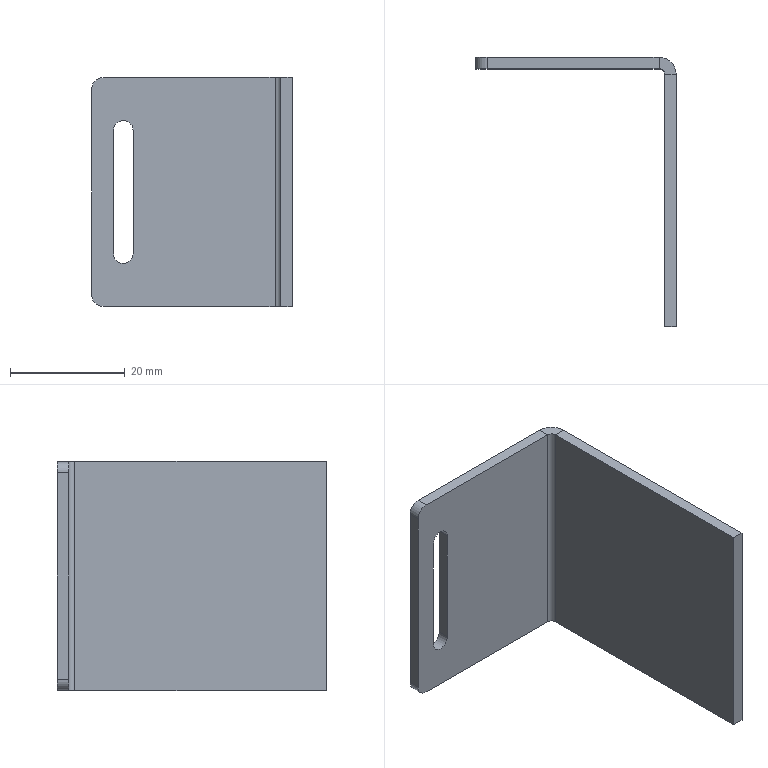Part | NX | features BREP 1 | 1 solid | 21 faces | box 35 x 47 x 40 mm | volume 6163 mm3 | plane 14 | cylinder 7 | commonest cylinder face diameters 3.4 x3 4 x2 2 x1 6 x1
STEP:
#1=CARTESIAN_POINT('',(2.,-2.,20.));
#2=VERTEX_POINT('',#1);
#3=CARTESIAN_POINT('',(0.,-2.,18.));
#4=VERTEX_POINT('',#3);
#5=CARTESIAN_POINT('',(2.,-2.,18.));
#6=DIRECTION('',(0.,-1.,0.));
#7=DIRECTION('',(0.,0.,1.));
#8=AXIS2_PLACEMENT_3D('',#5,#6,#7);
#9=CIRCLE('',#8,2.);
#10=EDGE_CURVE('',#2,#4,#9,.T.);
#11=ORIENTED_EDGE('',*,*,#10,.F.);
#12=CARTESIAN_POINT('',(2.,0.,20.));
#13=VERTEX_POINT('',#12);
#14=CARTESIAN_POINT('',(2.,-3.,20.));
#15=DIRECTION('',(0.,-1.,0.));
#16=VECTOR('',#15,1000.);
#17=LINE('',#14,#16);
#18=EDGE_CURVE('',#13,#2,#17,.T.);
#19=ORIENTED_EDGE('',*,*,#18,.F.);
#20=CARTESIAN_POINT('',(0.,0.,18.));
#21=VERTEX_POINT('',#20);
#22=CARTESIAN_POINT('',(2.,0.,18.));
#23=DIRECTION('',(0.,1.,0.));
#24=DIRECTION('',(0.,0.,1.));
#25=AXIS2_PLACEMENT_3D('',#22,#23,#24);
#26=CIRCLE('',#25,2.);
#27=EDGE_CURVE('',#21,#13,#26,.T.);
#28=ORIENTED_EDGE('',*,*,#27,.F.);
#29=CARTESIAN_POINT('',(0.,-2.,18.));
#30=DIRECTION('',(0.,1.,0.));
#31=VECTOR('',#30,1000.);
#32=LINE('',#29,#31);
#33=EDGE_CURVE('',#4,#21,#32,.T.);
#34=ORIENTED_EDGE('',*,*,#33,.F.);
#35=EDGE_LOOP('',(#11,#19,#28,#34));
#36=FACE_BOUND('',#35,.T.);
#37=CARTESIAN_POINT('',(2.,-2.,18.));
#38=DIRECTION('',(0.,1.,0.));
#39=DIRECTION('',(0.,0.,1.));
#40=AXIS2_PLACEMENT_3D('',#37,#38,#39);
#41=CYLINDRICAL_SURFACE('',#40,2.);
#42=ADVANCED_FACE('',(#36),#41,.T.);
#43=CARTESIAN_POINT('',(0.,-2.,-18.));
#44=VERTEX_POINT('',#43);
#45=CARTESIAN_POINT('',(2.,-2.,-20.));
#46=VERTEX_POINT('',#45);
#47=CARTESIAN_POINT('',(2.,-2.,-18.));
#48=DIRECTION('',(0.,-1.,0.));
#49=DIRECTION('',(0.,0.,1.));
#50=AXIS2_PLACEMENT_3D('',#47,#48,#49);
#51=CIRCLE('',#50,2.);
#52=EDGE_CURVE('',#44,#46,#51,.T.);
#53=ORIENTED_EDGE('',*,*,#52,.F.);
#54=CARTESIAN_POINT('',(0.,0.,-18.));
#55=VERTEX_POINT('',#54);
#56=CARTESIAN_POINT('',(0.,-2.,-18.));
#57=DIRECTION('',(0.,-1.,0.));
#58=VECTOR('',#57,1000.);
#59=LINE('',#56,#58);
#60=EDGE_CURVE('',#55,#44,#59,.T.);
#61=ORIENTED_EDGE('',*,*,#60,.F.);
#62=CARTESIAN_POINT('',(2.,0.,-20.));
#63=VERTEX_POINT('',#62);
#64=CARTESIAN_POINT('',(2.,0.,-18.));
#65=DIRECTION('',(0.,1.,0.));
#66=DIRECTION('',(0.,0.,1.));
#67=AXIS2_PLACEMENT_3D('',#64,#65,#66);
#68=CIRCLE('',#67,2.);
#69=EDGE_CURVE('',#63,#55,#68,.T.);
#70=ORIENTED_EDGE('',*,*,#69,.F.);
#71=CARTESIAN_POINT('',(2.,-3.,-20.));
#72=DIRECTION('',(0.,1.,0.));
#73=VECTOR('',#72,1000.);
#74=LINE('',#71,#73);
#75=EDGE_CURVE('',#46,#63,#74,.T.);
#76=ORIENTED_EDGE('',*,*,#75,.F.);
#77=EDGE_LOOP('',(#53,#61,#70,#76));
#78=FACE_BOUND('',#77,.T.);
#79=CARTESIAN_POINT('',(2.,-3.,-18.));
#80=DIRECTION('',(0.,1.,0.));
#81=DIRECTION('',(0.,0.,1.));
#82=AXIS2_PLACEMENT_3D('',#79,#80,#81);
#83=CYLINDRICAL_SURFACE('',#82,2.);
#84=ADVANCED_FACE('',(#78),#83,.T.);
#85=CARTESIAN_POINT('',(7.2,0.,-10.8));
#86=VERTEX_POINT('',#85);
#87=CARTESIAN_POINT('',(7.2,-2.,-10.8));
#88=VERTEX_POINT('',#87);
#89=CARTESIAN_POINT('',(7.2,-47.,-10.8));
#90=DIRECTION('',(0.,-1.,0.));
#91=VECTOR('',#90,1000.);
#92=LINE('',#89,#91);
#93=EDGE_CURVE('',#86,#88,#92,.T.);
#94=ORIENTED_EDGE('',*,*,#93,.F.);
#95=CARTESIAN_POINT('',(3.8,0.,-10.8));
#96=VERTEX_POINT('',#95);
#97=CARTESIAN_POINT('',(5.5,0.,-10.8));
#98=DIRECTION('',(0.,1.,0.));
#99=DIRECTION('',(0.,0.,1.));
#100=AXIS2_PLACEMENT_3D('',#97,#98,#99);
#101=CIRCLE('',#100,1.7);
#102=EDGE_CURVE('',#86,#96,#101,.T.);
#103=ORIENTED_EDGE('',*,*,#102,.T.);
#104=CARTESIAN_POINT('',(3.8,-2.,-10.8));
#105=VERTEX_POINT('',#104);
#106=CARTESIAN_POINT('',(3.8,0.,-10.8));
#107=DIRECTION('',(0.,1.,0.));
#108=VECTOR('',#107,1000.);
#109=LINE('',#106,#108);
#110=EDGE_CURVE('',#105,#96,#109,.T.);
#111=ORIENTED_EDGE('',*,*,#110,.F.);
#112=CARTESIAN_POINT('',(5.5,-2.,-10.8));
#113=DIRECTION('',(0.,1.,0.));
#114=DIRECTION('',(0.,0.,1.));
#115=AXIS2_PLACEMENT_3D('',#112,#113,#114);
#116=CIRCLE('',#115,1.7);
#117=EDGE_CURVE('',#88,#105,#116,.T.);
#118=ORIENTED_EDGE('',*,*,#117,.F.);
#119=EDGE_LOOP('',(#94,#103,#111,#118));
#120=FACE_BOUND('',#119,.T.);
#121=CARTESIAN_POINT('',(5.5,0.,-10.8));
#122=DIRECTION('',(0.,1.,0.));
#123=DIRECTION('',(0.,0.,1.));
#124=AXIS2_PLACEMENT_3D('',#121,#122,#123);
#125=CYLINDRICAL_SURFACE('',#124,1.7);
#126=ADVANCED_FACE('',(#120),#125,.F.);
#127=CARTESIAN_POINT('',(7.2,0.,10.8));
#128=VERTEX_POINT('',#127);
#129=CARTESIAN_POINT('',(7.2,-2.,10.8));
#130=VERTEX_POINT('',#129);
#131=CARTESIAN_POINT('',(7.2,-47.,10.8));
#132=DIRECTION('',(0.,-1.,0.));
#133=VECTOR('',#132,1000.);
#134=LINE('',#131,#133);
#135=EDGE_CURVE('',#128,#130,#134,.T.);
#136=ORIENTED_EDGE('',*,*,#135,.F.);
#137=CARTESIAN_POINT('',(7.2,0.,10.8));
#138=DIRECTION('',(0.,0.,-1.));
#139=VECTOR('',#138,1000.);
#140=LINE('',#137,#139);
#141=EDGE_CURVE('',#128,#86,#140,.T.);
#142=ORIENTED_EDGE('',*,*,#141,.T.);
#143=ORIENTED_EDGE('',*,*,#93,.T.);
#144=CARTESIAN_POINT('',(7.2,-2.,20.));
#145=DIRECTION('',(0.,0.,-1.));
#146=VECTOR('',#145,1000.);
#147=LINE('',#144,#146);
#148=EDGE_CURVE('',#130,#88,#147,.T.);
#149=ORIENTED_EDGE('',*,*,#148,.F.);
#150=EDGE_LOOP('',(#136,#142,#143,#149));
#151=FACE_BOUND('',#150,.T.);
#152=CARTESIAN_POINT('',(7.2,-47.,10.8));
#153=DIRECTION('',(1.,0.,0.));
#154=DIRECTION('',(0.,1.,0.));
#155=AXIS2_PLACEMENT_3D('',#152,#153,#154);
#156=PLANE('',#155);
#157=ADVANCED_FACE('',(#151),#156,.F.);
#158=CARTESIAN_POINT('',(5.5,-2.,12.5));
#159=VERTEX_POINT('',#158);
#160=CARTESIAN_POINT('',(5.5,0.,12.5));
#161=VERTEX_POINT('',#160);
#162=CARTESIAN_POINT('',(5.5,0.,12.5));
#163=DIRECTION('',(0.,1.,0.));
#164=VECTOR('',#163,1000.);
#165=LINE('',#162,#164);
#166=EDGE_CURVE('',#159,#161,#165,.T.);
#167=ORIENTED_EDGE('',*,*,#166,.F.);
#168=CARTESIAN_POINT('',(3.8,-2.,10.8));
#169=VERTEX_POINT('',#168);
#170=CARTESIAN_POINT('',(5.5,-2.,10.8));
#171=DIRECTION('',(0.,1.,0.));
#172=DIRECTION('',(0.,0.,1.));
#173=AXIS2_PLACEMENT_3D('',#170,#171,#172);
#174=CIRCLE('',#173,1.7);
#175=EDGE_CURVE('',#169,#159,#174,.T.);
#176=ORIENTED_EDGE('',*,*,#175,.F.);
#177=CARTESIAN_POINT('',(3.8,0.,10.8));
#178=VERTEX_POINT('',#177);
#179=CARTESIAN_POINT('',(3.8,0.,10.8));
#180=DIRECTION('',(0.,-1.,0.));
#181=VECTOR('',#180,1000.);
#182=LINE('',#179,#181);
#183=EDGE_CURVE('',#178,#169,#182,.T.);
#184=ORIENTED_EDGE('',*,*,#183,.F.);
#185=CARTESIAN_POINT('',(5.5,0.,10.8));
#186=DIRECTION('',(0.,1.,0.));
#187=DIRECTION('',(0.,0.,1.));
#188=AXIS2_PLACEMENT_3D('',#185,#186,#187);
#189=CIRCLE('',#188,1.7);
#190=EDGE_CURVE('',#178,#161,#189,.T.);
#191=ORIENTED_EDGE('',*,*,#190,.T.);
#192=EDGE_LOOP('',(#167,#176,#184,#191));
#193=FACE_BOUND('',#192,.T.);
#194=CARTESIAN_POINT('',(5.5,0.,10.8));
#195=DIRECTION('',(0.,1.,0.));
#196=DIRECTION('',(0.,0.,1.));
#197=AXIS2_PLACEMENT_3D('',#194,#195,#196);
#198=CYLINDRICAL_SURFACE('',#197,1.7);
#199=ADVANCED_FACE('',(#193),#198,.F.);
#200=ORIENTED_EDGE('',*,*,#110,.T.);
#201=CARTESIAN_POINT('',(3.8,0.,10.8));
#202=DIRECTION('',(0.,0.,-1.));
#203=VECTOR('',#202,1000.);
#204=LINE('',#201,#203);
#205=EDGE_CURVE('',#178,#96,#204,.T.);
#206=ORIENTED_EDGE('',*,*,#205,.F.);
#207=ORIENTED_EDGE('',*,*,#183,.T.);
#208=CARTESIAN_POINT('',(3.8,-2.,20.));
#209=DIRECTION('',(0.,0.,1.));
#210=VECTOR('',#209,1000.);
#211=LINE('',#208,#210);
#212=EDGE_CURVE('',#105,#169,#211,.T.);
#213=ORIENTED_EDGE('',*,*,#212,.F.);
#214=EDGE_LOOP('',(#200,#206,#207,#213));
#215=FACE_BOUND('',#214,.T.);
#216=CARTESIAN_POINT('',(3.8,0.,10.8));
#217=DIRECTION('',(-1.,0.,0.));
#218=DIRECTION('',(0.,0.,1.));
#219=AXIS2_PLACEMENT_3D('',#216,#217,#218);
#220=PLANE('',#219);
#221=ADVANCED_FACE('',(#215),#220,.F.);
#222=CARTESIAN_POINT('',(33.,-3.,-20.));
#223=VERTEX_POINT('',#222);
#224=CARTESIAN_POINT('',(33.,-47.,-20.));
#225=VERTEX_POINT('',#224);
#226=CARTESIAN_POINT('',(33.,0.,-20.));
#227=DIRECTION('',(0.,-1.,0.));
#228=VECTOR('',#227,1000.);
#229=LINE('',#226,#228);
#230=EDGE_CURVE('',#223,#225,#229,.T.);
#231=ORIENTED_EDGE('',*,*,#230,.F.);
#232=CARTESIAN_POINT('',(35.,-3.,-20.));
#233=VERTEX_POINT('',#232);
#234=CARTESIAN_POINT('',(33.,-3.,-20.));
#235=DIRECTION('',(1.,0.,0.));
#236=VECTOR('',#235,1000.);
#237=LINE('',#234,#236);
#238=EDGE_CURVE('',#223,#233,#237,.T.);
#239=ORIENTED_EDGE('',*,*,#238,.T.);
#240=CARTESIAN_POINT('',(35.,-47.,-20.));
#241=VERTEX_POINT('',#240);
#242=CARTESIAN_POINT('',(35.,0.,-20.));
#243=DIRECTION('',(0.,-1.,0.));
#244=VECTOR('',#243,1000.);
#245=LINE('',#242,#244);
#246=EDGE_CURVE('',#233,#241,#245,.T.);
#247=ORIENTED_EDGE('',*,*,#246,.T.);
#248=CARTESIAN_POINT('',(35.,-47.,-20.));
#249=DIRECTION('',(-1.,0.,0.));
#250=VECTOR('',#249,1000.);
#251=LINE('',#248,#250);
#252=EDGE_CURVE('',#241,#225,#251,.T.);
#253=ORIENTED_EDGE('',*,*,#252,.T.);
#254=EDGE_LOOP('',(#231,#239,#247,#253));
#255=FACE_BOUND('',#254,.T.);
#256=CARTESIAN_POINT('',(32.,-3.,-20.));
#257=DIRECTION('',(0.,0.,1.));
#258=DIRECTION('',(1.,0.,0.));
#259=AXIS2_PLACEMENT_3D('',#256,#257,#258);
#260=PLANE('',#259);
#261=ADVANCED_FACE('',(#255),#260,.F.);
#262=CARTESIAN_POINT('',(32.,0.,20.));
#263=VERTEX_POINT('',#262);
#264=CARTESIAN_POINT('',(0.,0.,20.));
#265=DIRECTION('',(1.,0.,0.));
#266=VECTOR('',#265,1000.);
#267=LINE('',#264,#266);
#268=EDGE_CURVE('',#13,#263,#267,.T.);
#269=ORIENTED_EDGE('',*,*,#268,.F.);
#270=ORIENTED_EDGE('',*,*,#18,.T.);
#271=CARTESIAN_POINT('',(32.,-2.,20.));
#272=VERTEX_POINT('',#271);
#273=CARTESIAN_POINT('',(0.,-2.,20.));
#274=DIRECTION('',(1.,0.,0.));
#275=VECTOR('',#274,1000.);
#276=LINE('',#273,#275);
#277=EDGE_CURVE('',#2,#272,#276,.T.);
#278=ORIENTED_EDGE('',*,*,#277,.T.);
#279=CARTESIAN_POINT('',(32.,-2.,20.));
#280=DIRECTION('',(0.,1.,0.));
#281=VECTOR('',#280,1000.);
#282=LINE('',#279,#281);
#283=EDGE_CURVE('',#272,#263,#282,.T.);
#284=ORIENTED_EDGE('',*,*,#283,.T.);
#285=EDGE_LOOP('',(#269,#270,#278,#284));
#286=FACE_BOUND('',#285,.T.);
#287=CARTESIAN_POINT('',(32.,-3.,20.));
#288=DIRECTION('',(0.,0.,1.));
#289=DIRECTION('',(1.,0.,0.));
#290=AXIS2_PLACEMENT_3D('',#287,#288,#289);
#291=PLANE('',#290);
#292=ADVANCED_FACE('',(#286),#291,.T.);
#293=CARTESIAN_POINT('',(32.,-2.,-20.));
#294=VERTEX_POINT('',#293);
#295=CARTESIAN_POINT('',(32.,-3.,-20.));
#296=DIRECTION('',(0.,0.,-1.));
#297=DIRECTION('',(1.,0.,0.));
#298=AXIS2_PLACEMENT_3D('',#295,#296,#297);
#299=CIRCLE('',#298,1.);
#300=EDGE_CURVE('',#294,#223,#299,.T.);
#301=ORIENTED_EDGE('',*,*,#300,.T.);
#302=CARTESIAN_POINT('',(33.,-3.,20.));
#303=VERTEX_POINT('',#302);
#304=CARTESIAN_POINT('',(33.,-3.,20.));
#305=DIRECTION('',(0.,0.,-1.));
#306=VECTOR('',#305,1000.);
#307=LINE('',#304,#306);
#308=EDGE_CURVE('',#303,#223,#307,.T.);
#309=ORIENTED_EDGE('',*,*,#308,.F.);
#310=CARTESIAN_POINT('',(32.,-3.,20.));
#311=DIRECTION('',(0.,0.,-1.));
#312=DIRECTION('',(1.,0.,0.));
#313=AXIS2_PLACEMENT_3D('',#310,#311,#312);
#314=CIRCLE('',#313,1.);
#315=EDGE_CURVE('',#272,#303,#314,.T.);
#316=ORIENTED_EDGE('',*,*,#315,.F.);
#317=CARTESIAN_POINT('',(32.,-2.,20.));
#318=DIRECTION('',(0.,0.,-1.));
#319=VECTOR('',#318,1000.);
#320=LINE('',#317,#319);
#321=EDGE_CURVE('',#272,#294,#320,.T.);
#322=ORIENTED_EDGE('',*,*,#321,.T.);
#323=EDGE_LOOP('',(#301,#309,#316,#322));
#324=FACE_BOUND('',#323,.T.);
#325=CARTESIAN_POINT('',(32.,-3.,20.));
#326=DIRECTION('',(0.,0.,-1.));
#327=DIRECTION('',(-1.,0.,0.));
#328=AXIS2_PLACEMENT_3D('',#325,#326,#327);
#329=CYLINDRICAL_SURFACE('',#328,1.);
#330=ADVANCED_FACE('',(#324),#329,.F.);
#331=CARTESIAN_POINT('',(0.,-2.,20.));
#332=DIRECTION('',(0.,0.,-1.));
#333=VECTOR('',#332,1000.);
#334=LINE('',#331,#333);
#335=EDGE_CURVE('',#4,#44,#334,.T.);
#336=ORIENTED_EDGE('',*,*,#335,.T.);
#337=ORIENTED_EDGE('',*,*,#52,.T.);
#338=CARTESIAN_POINT('',(0.,-2.,-20.));
#339=DIRECTION('',(1.,0.,0.));
#340=VECTOR('',#339,1000.);
#341=LINE('',#338,#340);
#342=EDGE_CURVE('',#46,#294,#341,.T.);
#343=ORIENTED_EDGE('',*,*,#342,.T.);
#344=ORIENTED_EDGE('',*,*,#321,.F.);
#345=ORIENTED_EDGE('',*,*,#277,.F.);
#346=ORIENTED_EDGE('',*,*,#10,.T.);
#347=EDGE_LOOP('',(#336,#337,#343,#344,#345,#346));
#348=FACE_BOUND('',#347,.T.);
#349=ORIENTED_EDGE('',*,*,#212,.T.);
#350=ORIENTED_EDGE('',*,*,#175,.T.);
#351=CARTESIAN_POINT('',(5.5,-2.,10.8));
#352=DIRECTION('',(0.,1.,0.));
#353=DIRECTION('',(0.,0.,1.));
#354=AXIS2_PLACEMENT_3D('',#351,#352,#353);
#355=CIRCLE('',#354,1.7);
#356=EDGE_CURVE('',#159,#130,#355,.T.);
#357=ORIENTED_EDGE('',*,*,#356,.T.);
#358=ORIENTED_EDGE('',*,*,#148,.T.);
#359=ORIENTED_EDGE('',*,*,#117,.T.);
#360=EDGE_LOOP('',(#349,#350,#357,#358,#359));
#361=FACE_BOUND('',#360,.T.);
#362=CARTESIAN_POINT('',(0.,-2.,20.));
#363=DIRECTION('',(0.,1.,0.));
#364=DIRECTION('',(0.,0.,1.));
#365=AXIS2_PLACEMENT_3D('',#362,#363,#364);
#366=PLANE('',#365);
#367=ADVANCED_FACE('',(#348,#361),#366,.F.);
#368=CARTESIAN_POINT('',(0.,0.,20.));
#369=DIRECTION('',(0.,0.,-1.));
#370=VECTOR('',#369,1000.);
#371=LINE('',#368,#370);
#372=EDGE_CURVE('',#21,#55,#371,.T.);
#373=ORIENTED_EDGE('',*,*,#372,.T.);
#374=ORIENTED_EDGE('',*,*,#60,.T.);
#375=ORIENTED_EDGE('',*,*,#335,.F.);
#376=ORIENTED_EDGE('',*,*,#33,.T.);
#377=EDGE_LOOP('',(#373,#374,#375,#376));
#378=FACE_BOUND('',#377,.T.);
#379=CARTESIAN_POINT('',(0.,-2.,20.));
#380=DIRECTION('',(-1.,0.,0.));
#381=DIRECTION('',(0.,0.,1.));
#382=AXIS2_PLACEMENT_3D('',#379,#380,#381);
#383=PLANE('',#382);
#384=ADVANCED_FACE('',(#378),#383,.T.);
#385=CARTESIAN_POINT('',(32.,0.,-20.));
#386=VERTEX_POINT('',#385);
#387=CARTESIAN_POINT('',(0.,0.,-20.));
#388=DIRECTION('',(1.,0.,0.));
#389=VECTOR('',#388,1000.);
#390=LINE('',#387,#389);
#391=EDGE_CURVE('',#63,#386,#390,.T.);
#392=ORIENTED_EDGE('',*,*,#391,.F.);
#393=ORIENTED_EDGE('',*,*,#69,.T.);
#394=ORIENTED_EDGE('',*,*,#372,.F.);
#395=ORIENTED_EDGE('',*,*,#27,.T.);
#396=ORIENTED_EDGE('',*,*,#268,.T.);
#397=CARTESIAN_POINT('',(32.,0.,20.));
#398=DIRECTION('',(0.,0.,-1.));
#399=VECTOR('',#398,1000.);
#400=LINE('',#397,#399);
#401=EDGE_CURVE('',#263,#386,#400,.T.);
#402=ORIENTED_EDGE('',*,*,#401,.T.);
#403=EDGE_LOOP('',(#392,#393,#394,#395,#396,#402));
#404=FACE_BOUND('',#403,.T.);
#405=ORIENTED_EDGE('',*,*,#205,.T.);
#406=ORIENTED_EDGE('',*,*,#102,.F.);
#407=ORIENTED_EDGE('',*,*,#141,.F.);
#408=CARTESIAN_POINT('',(5.5,0.,10.8));
#409=DIRECTION('',(0.,1.,0.));
#410=DIRECTION('',(0.,0.,1.));
#411=AXIS2_PLACEMENT_3D('',#408,#409,#410);
#412=CIRCLE('',#411,1.7);
#413=EDGE_CURVE('',#161,#128,#412,.T.);
#414=ORIENTED_EDGE('',*,*,#413,.F.);
#415=ORIENTED_EDGE('',*,*,#190,.F.);
#416=EDGE_LOOP('',(#405,#406,#407,#414,#415));
#417=FACE_BOUND('',#416,.T.);
#418=CARTESIAN_POINT('',(0.,0.,20.));
#419=DIRECTION('',(0.,1.,0.));
#420=DIRECTION('',(0.,0.,1.));
#421=AXIS2_PLACEMENT_3D('',#418,#419,#420);
#422=PLANE('',#421);
#423=ADVANCED_FACE('',(#404,#417),#422,.T.);
#424=CARTESIAN_POINT('',(32.,-3.,-20.));
#425=DIRECTION('',(0.,0.,-1.));
#426=DIRECTION('',(1.,0.,0.));
#427=AXIS2_PLACEMENT_3D('',#424,#425,#426);
#428=CIRCLE('',#427,3.);
#429=EDGE_CURVE('',#386,#233,#428,.T.);
#430=ORIENTED_EDGE('',*,*,#429,.F.);
#431=ORIENTED_EDGE('',*,*,#401,.F.);
#432=CARTESIAN_POINT('',(35.,-3.,20.));
#433=VERTEX_POINT('',#432);
#434=CARTESIAN_POINT('',(32.,-3.,20.));
#435=DIRECTION('',(0.,0.,-1.));
#436=DIRECTION('',(1.,0.,0.));
#437=AXIS2_PLACEMENT_3D('',#434,#435,#436);
#438=CIRCLE('',#437,3.);
#439=EDGE_CURVE('',#263,#433,#438,.T.);
#440=ORIENTED_EDGE('',*,*,#439,.T.);
#441=CARTESIAN_POINT('',(35.,-3.,20.));
#442=DIRECTION('',(0.,0.,-1.));
#443=VECTOR('',#442,1000.);
#444=LINE('',#441,#443);
#445=EDGE_CURVE('',#433,#233,#444,.T.);
#446=ORIENTED_EDGE('',*,*,#445,.T.);
#447=EDGE_LOOP('',(#430,#431,#440,#446));
#448=FACE_BOUND('',#447,.T.);
#449=CARTESIAN_POINT('',(32.,-3.,20.));
#450=DIRECTION('',(0.,0.,-1.));
#451=DIRECTION('',(-1.,0.,0.));
#452=AXIS2_PLACEMENT_3D('',#449,#450,#451);
#453=CYLINDRICAL_SURFACE('',#452,3.);
#454=ADVANCED_FACE('',(#448),#453,.T.);
#455=ORIENTED_EDGE('',*,*,#246,.F.);
#456=ORIENTED_EDGE('',*,*,#445,.F.);
#457=CARTESIAN_POINT('',(35.,-47.,20.));
#458=VERTEX_POINT('',#457);
#459=CARTESIAN_POINT('',(35.,0.,20.));
#460=DIRECTION('',(0.,-1.,0.));
#461=VECTOR('',#460,1000.);
#462=LINE('',#459,#461);
#463=EDGE_CURVE('',#433,#458,#462,.T.);
#464=ORIENTED_EDGE('',*,*,#463,.T.);
#465=CARTESIAN_POINT('',(35.,-47.,20.));
#466=DIRECTION('',(0.,0.,-1.));
#467=VECTOR('',#466,1000.);
#468=LINE('',#465,#467);
#469=EDGE_CURVE('',#458,#241,#468,.T.);
#470=ORIENTED_EDGE('',*,*,#469,.T.);
#471=EDGE_LOOP('',(#455,#456,#464,#470));
#472=FACE_BOUND('',#471,.T.);
#473=CARTESIAN_POINT('',(35.,0.,20.));
#474=DIRECTION('',(1.,0.,0.));
#475=DIRECTION('',(0.,1.,0.));
#476=AXIS2_PLACEMENT_3D('',#473,#474,#475);
#477=PLANE('',#476);
#478=ADVANCED_FACE('',(#472),#477,.T.);
#479=ORIENTED_EDGE('',*,*,#252,.F.);
#480=ORIENTED_EDGE('',*,*,#469,.F.);
#481=CARTESIAN_POINT('',(33.,-47.,20.));
#482=VERTEX_POINT('',#481);
#483=CARTESIAN_POINT('',(35.,-47.,20.));
#484=DIRECTION('',(-1.,0.,0.));
#485=VECTOR('',#484,1000.);
#486=LINE('',#483,#485);
#487=EDGE_CURVE('',#458,#482,#486,.T.);
#488=ORIENTED_EDGE('',*,*,#487,.T.);
#489=CARTESIAN_POINT('',(33.,-47.,20.));
#490=DIRECTION('',(0.,0.,-1.));
#491=VECTOR('',#490,1000.);
#492=LINE('',#489,#491);
#493=EDGE_CURVE('',#482,#225,#492,.T.);
#494=ORIENTED_EDGE('',*,*,#493,.T.);
#495=EDGE_LOOP('',(#479,#480,#488,#494));
#496=FACE_BOUND('',#495,.T.);
#497=CARTESIAN_POINT('',(35.,-47.,20.));
#498=DIRECTION('',(0.,-1.,0.));
#499=DIRECTION('',(0.,0.,-1.));
#500=AXIS2_PLACEMENT_3D('',#497,#498,#499);
#501=PLANE('',#500);
#502=ADVANCED_FACE('',(#496),#501,.T.);
#503=ORIENTED_EDGE('',*,*,#230,.T.);
#504=ORIENTED_EDGE('',*,*,#493,.F.);
#505=CARTESIAN_POINT('',(33.,0.,20.));
#506=DIRECTION('',(0.,-1.,0.));
#507=VECTOR('',#506,1000.);
#508=LINE('',#505,#507);
#509=EDGE_CURVE('',#303,#482,#508,.T.);
#510=ORIENTED_EDGE('',*,*,#509,.F.);
#511=ORIENTED_EDGE('',*,*,#308,.T.);
#512=EDGE_LOOP('',(#503,#504,#510,#511));
#513=FACE_BOUND('',#512,.T.);
#514=CARTESIAN_POINT('',(33.,0.,20.));
#515=DIRECTION('',(1.,0.,0.));
#516=DIRECTION('',(0.,1.,0.));
#517=AXIS2_PLACEMENT_3D('',#514,#515,#516);
#518=PLANE('',#517);
#519=ADVANCED_FACE('',(#513),#518,.F.);
#520=ORIENTED_EDGE('',*,*,#342,.F.);
#521=ORIENTED_EDGE('',*,*,#75,.T.);
#522=ORIENTED_EDGE('',*,*,#391,.T.);
#523=CARTESIAN_POINT('',(32.,0.,-20.));
#524=DIRECTION('',(0.,-1.,0.));
#525=VECTOR('',#524,1000.);
#526=LINE('',#523,#525);
#527=EDGE_CURVE('',#386,#294,#526,.T.);
#528=ORIENTED_EDGE('',*,*,#527,.T.);
#529=EDGE_LOOP('',(#520,#521,#522,#528));
#530=FACE_BOUND('',#529,.T.);
#531=CARTESIAN_POINT('',(33.,-3.,-20.));
#532=DIRECTION('',(0.,0.,-1.));
#533=DIRECTION('',(-1.,0.,0.));
#534=AXIS2_PLACEMENT_3D('',#531,#532,#533);
#535=PLANE('',#534);
#536=ADVANCED_FACE('',(#530),#535,.T.);
#537=ORIENTED_EDGE('',*,*,#527,.F.);
#538=ORIENTED_EDGE('',*,*,#429,.T.);
#539=ORIENTED_EDGE('',*,*,#238,.F.);
#540=ORIENTED_EDGE('',*,*,#300,.F.);
#541=EDGE_LOOP('',(#537,#538,#539,#540));
#542=FACE_BOUND('',#541,.T.);
#543=CARTESIAN_POINT('',(32.,0.,-20.));
#544=DIRECTION('',(0.,0.,-1.));
#545=DIRECTION('',(-1.,0.,0.));
#546=AXIS2_PLACEMENT_3D('',#543,#544,#545);
#547=PLANE('',#546);
#548=ADVANCED_FACE('',(#542),#547,.T.);
#549=ORIENTED_EDGE('',*,*,#463,.F.);
#550=CARTESIAN_POINT('',(35.,-3.,20.));
#551=DIRECTION('',(-1.,0.,0.));
#552=VECTOR('',#551,1000.);
#553=LINE('',#550,#552);
#554=EDGE_CURVE('',#433,#303,#553,.T.);
#555=ORIENTED_EDGE('',*,*,#554,.T.);
#556=ORIENTED_EDGE('',*,*,#509,.T.);
#557=ORIENTED_EDGE('',*,*,#487,.F.);
#558=EDGE_LOOP('',(#549,#555,#556,#557));
#559=FACE_BOUND('',#558,.T.);
#560=CARTESIAN_POINT('',(32.,-2.,20.));
#561=DIRECTION('',(0.,0.,1.));
#562=DIRECTION('',(1.,0.,0.));
#563=AXIS2_PLACEMENT_3D('',#560,#561,#562);
#564=PLANE('',#563);
#565=ADVANCED_FACE('',(#559),#564,.T.);
#566=ORIENTED_EDGE('',*,*,#554,.F.);
#567=ORIENTED_EDGE('',*,*,#439,.F.);
#568=ORIENTED_EDGE('',*,*,#283,.F.);
#569=ORIENTED_EDGE('',*,*,#315,.T.);
#570=EDGE_LOOP('',(#566,#567,#568,#569));
#571=FACE_BOUND('',#570,.T.);
#572=CARTESIAN_POINT('',(35.,-3.,20.));
#573=DIRECTION('',(0.,0.,1.));
#574=DIRECTION('',(1.,0.,0.));
#575=AXIS2_PLACEMENT_3D('',#572,#573,#574);
#576=PLANE('',#575);
#577=ADVANCED_FACE('',(#571),#576,.T.);
#578=ORIENTED_EDGE('',*,*,#356,.F.);
#579=ORIENTED_EDGE('',*,*,#166,.T.);
#580=ORIENTED_EDGE('',*,*,#413,.T.);
#581=ORIENTED_EDGE('',*,*,#135,.T.);
#582=EDGE_LOOP('',(#578,#579,#580,#581));
#583=FACE_BOUND('',#582,.T.);
#584=CARTESIAN_POINT('',(5.5,0.,10.8));
#585=DIRECTION('',(0.,1.,0.));
#586=DIRECTION('',(0.,0.,1.));
#587=AXIS2_PLACEMENT_3D('',#584,#585,#586);
#588=CYLINDRICAL_SURFACE('',#587,1.7);
#589=ADVANCED_FACE('',(#583),#588,.F.);
#590=CLOSED_SHELL('',(#42,#84,#126,#157,#199,#221,#261,#292,#330,#367,#384,#423,#454,#478,#502,#519,#536,#548,#565,#577,#589));
#591=MANIFOLD_SOLID_BREP('',#590);
#592=(LENGTH_UNIT()NAMED_UNIT(*)SI_UNIT(.MILLI.,.METRE.));
#593=UNCERTAINTY_MEASURE_WITH_UNIT(LENGTH_MEASURE(0.00001),#592,'','');
#594=(NAMED_UNIT(*)PLANE_ANGLE_UNIT()SI_UNIT($,.RADIAN.));
#595=(NAMED_UNIT(*)SI_UNIT($,.STERADIAN.)SOLID_ANGLE_UNIT());
#596=(GEOMETRIC_REPRESENTATION_CONTEXT(3)GLOBAL_UNCERTAINTY_ASSIGNED_CONTEXT((#593))GLOBAL_UNIT_ASSIGNED_CONTEXT((#592,#594,#595))REPRESENTATION_CONTEXT('',''));
#597=ADVANCED_BREP_SHAPE_REPRESENTATION('',(#591),#596);